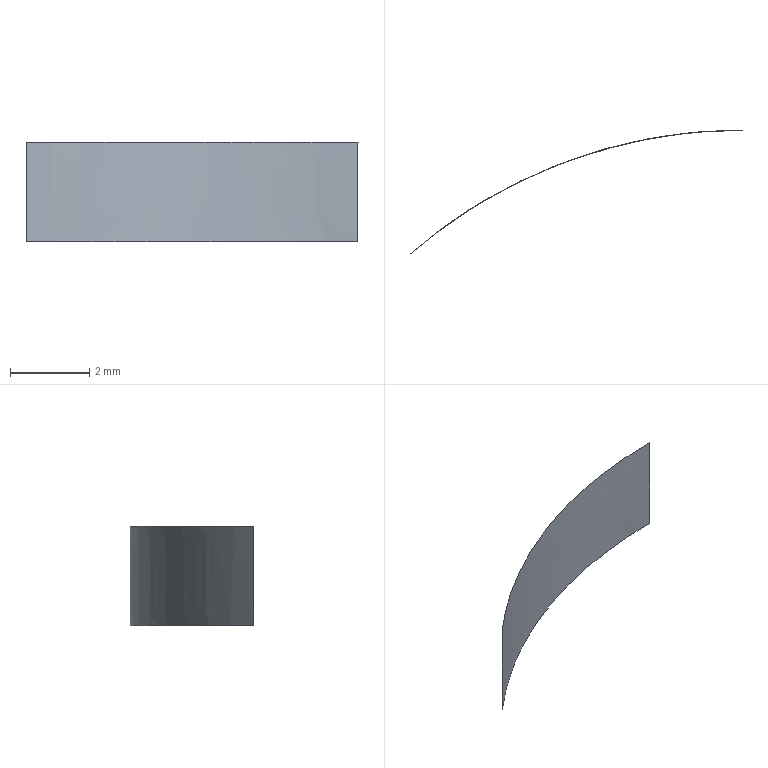Part | STEP file | lll_id378_x_t | 1 solid | 2 faces | box 8.381 x 3.125 x 2.5 mm | volume 0.0177 mm3 | other 1 | cylinder 1 | commonest cylinder face diameters 25.6 x1